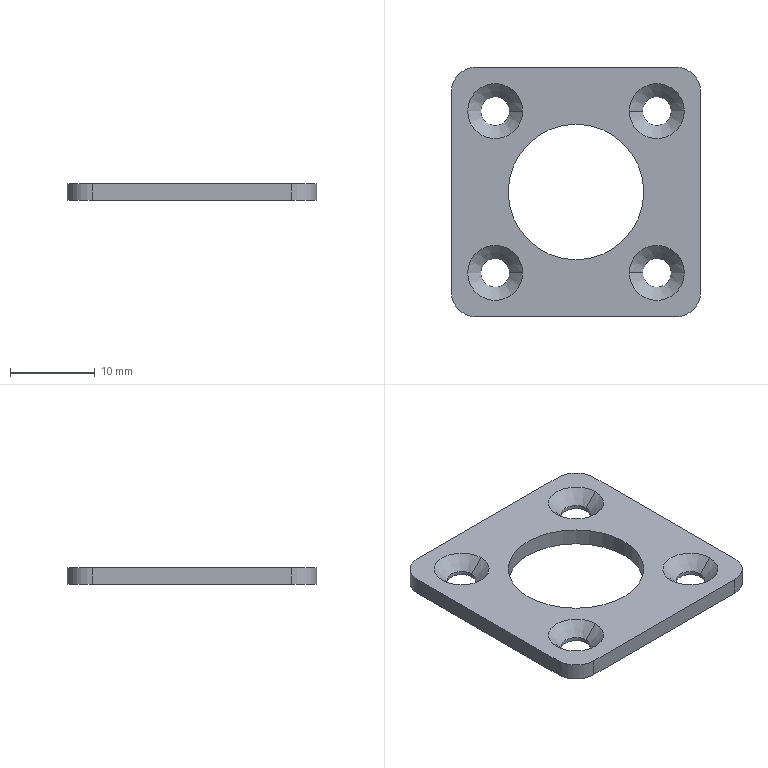Part | NX | features BREP 1 | 1 solid | 28 faces | box 29.5 x 29.5 x 2 mm | volume 1183 mm3 | cylinder 14 | cone 8 | plane 6 | commonest cylinder face diameters 3.4 x8 6 x4 16 x2
STEP:
#1=CARTESIAN_POINT('',(6.296,9.546,2.));
#2=VERTEX_POINT('',#1);
#3=CARTESIAN_POINT('',(7.846,9.546,0.45));
#4=VERTEX_POINT('',#3);
#5=CARTESIAN_POINT('',(6.296,9.546,2.));
#6=DIRECTION('',(-0.7071,0.,0.7071));
#7=VECTOR('',#6,1000.);
#8=LINE('',#5,#7);
#9=EDGE_CURVE('',#2,#4,#8,.F.);
#10=ORIENTED_EDGE('',*,*,#9,.T.);
#11=CARTESIAN_POINT('',(11.246,9.546,0.45));
#12=VERTEX_POINT('',#11);
#13=CARTESIAN_POINT('',(9.546,9.546,0.45));
#14=DIRECTION('',(0.,0.,1.));
#15=DIRECTION('',(1.,0.,0.));
#16=AXIS2_PLACEMENT_3D('',#13,#14,#15);
#17=CIRCLE('',#16,1.7);
#18=EDGE_CURVE('',#12,#4,#17,.T.);
#19=ORIENTED_EDGE('',*,*,#18,.F.);
#20=CARTESIAN_POINT('',(12.796,9.546,2.));
#21=VERTEX_POINT('',#20);
#22=CARTESIAN_POINT('',(12.796,9.546,2.));
#23=DIRECTION('',(0.7071,0.,0.7071));
#24=VECTOR('',#23,1000.);
#25=LINE('',#22,#24);
#26=EDGE_CURVE('',#21,#12,#25,.F.);
#27=ORIENTED_EDGE('',*,*,#26,.F.);
#28=CARTESIAN_POINT('',(9.546,9.546,2.));
#29=DIRECTION('',(0.,0.,1.));
#30=DIRECTION('',(1.,0.,0.));
#31=AXIS2_PLACEMENT_3D('',#28,#29,#30);
#32=CIRCLE('',#31,3.25);
#33=EDGE_CURVE('',#21,#2,#32,.T.);
#34=ORIENTED_EDGE('',*,*,#33,.T.);
#35=EDGE_LOOP('',(#10,#19,#27,#34));
#36=FACE_BOUND('',#35,.T.);
#37=CARTESIAN_POINT('',(9.546,9.546,2.));
#38=DIRECTION('',(0.,0.,1.));
#39=DIRECTION('',(1.,0.,0.));
#40=AXIS2_PLACEMENT_3D('',#37,#38,#39);
#41=CONICAL_SURFACE('',#40,3.25,0.7854);
#42=ADVANCED_FACE('',(#36),#41,.F.);
#43=CARTESIAN_POINT('',(7.846,9.546,0.));
#44=VERTEX_POINT('',#43);
#45=CARTESIAN_POINT('',(7.846,9.546,2.));
#46=DIRECTION('',(0.,0.,1.));
#47=VECTOR('',#46,1000.);
#48=LINE('',#45,#47);
#49=EDGE_CURVE('',#4,#44,#48,.F.);
#50=ORIENTED_EDGE('',*,*,#49,.T.);
#51=CARTESIAN_POINT('',(11.246,9.546,0.));
#52=VERTEX_POINT('',#51);
#53=CARTESIAN_POINT('',(9.546,9.546,0.));
#54=DIRECTION('',(0.,0.,-1.));
#55=DIRECTION('',(-1.,0.,0.));
#56=AXIS2_PLACEMENT_3D('',#53,#54,#55);
#57=CIRCLE('',#56,1.7);
#58=EDGE_CURVE('',#44,#52,#57,.T.);
#59=ORIENTED_EDGE('',*,*,#58,.T.);
#60=CARTESIAN_POINT('',(11.246,9.546,2.));
#61=DIRECTION('',(0.,0.,1.));
#62=VECTOR('',#61,1000.);
#63=LINE('',#60,#62);
#64=EDGE_CURVE('',#12,#52,#63,.F.);
#65=ORIENTED_EDGE('',*,*,#64,.F.);
#66=ORIENTED_EDGE('',*,*,#18,.T.);
#67=EDGE_LOOP('',(#50,#59,#65,#66));
#68=FACE_BOUND('',#67,.T.);
#69=CARTESIAN_POINT('',(9.546,9.546,2.));
#70=DIRECTION('',(0.,0.,1.));
#71=DIRECTION('',(1.,0.,0.));
#72=AXIS2_PLACEMENT_3D('',#69,#70,#71);
#73=CYLINDRICAL_SURFACE('',#72,1.7);
#74=ADVANCED_FACE('',(#68),#73,.F.);
#75=CARTESIAN_POINT('',(6.296,-9.546,2.));
#76=VERTEX_POINT('',#75);
#77=CARTESIAN_POINT('',(7.846,-9.546,0.45));
#78=VERTEX_POINT('',#77);
#79=CARTESIAN_POINT('',(6.296,-9.546,2.));
#80=DIRECTION('',(-0.7071,0.,0.7071));
#81=VECTOR('',#80,1000.);
#82=LINE('',#79,#81);
#83=EDGE_CURVE('',#76,#78,#82,.F.);
#84=ORIENTED_EDGE('',*,*,#83,.T.);
#85=CARTESIAN_POINT('',(11.246,-9.546,0.45));
#86=VERTEX_POINT('',#85);
#87=CARTESIAN_POINT('',(9.546,-9.546,0.45));
#88=DIRECTION('',(0.,0.,1.));
#89=DIRECTION('',(1.,0.,0.));
#90=AXIS2_PLACEMENT_3D('',#87,#88,#89);
#91=CIRCLE('',#90,1.7);
#92=EDGE_CURVE('',#86,#78,#91,.T.);
#93=ORIENTED_EDGE('',*,*,#92,.F.);
#94=CARTESIAN_POINT('',(12.796,-9.546,2.));
#95=VERTEX_POINT('',#94);
#96=CARTESIAN_POINT('',(12.796,-9.546,2.));
#97=DIRECTION('',(0.7071,0.,0.7071));
#98=VECTOR('',#97,1000.);
#99=LINE('',#96,#98);
#100=EDGE_CURVE('',#95,#86,#99,.F.);
#101=ORIENTED_EDGE('',*,*,#100,.F.);
#102=CARTESIAN_POINT('',(9.546,-9.546,2.));
#103=DIRECTION('',(0.,0.,1.));
#104=DIRECTION('',(1.,0.,0.));
#105=AXIS2_PLACEMENT_3D('',#102,#103,#104);
#106=CIRCLE('',#105,3.25);
#107=EDGE_CURVE('',#95,#76,#106,.T.);
#108=ORIENTED_EDGE('',*,*,#107,.T.);
#109=EDGE_LOOP('',(#84,#93,#101,#108));
#110=FACE_BOUND('',#109,.T.);
#111=CARTESIAN_POINT('',(9.546,-9.546,2.));
#112=DIRECTION('',(0.,0.,1.));
#113=DIRECTION('',(1.,0.,0.));
#114=AXIS2_PLACEMENT_3D('',#111,#112,#113);
#115=CONICAL_SURFACE('',#114,3.25,0.7854);
#116=ADVANCED_FACE('',(#110),#115,.F.);
#117=CARTESIAN_POINT('',(7.846,-9.546,0.));
#118=VERTEX_POINT('',#117);
#119=CARTESIAN_POINT('',(7.846,-9.546,2.));
#120=DIRECTION('',(0.,0.,1.));
#121=VECTOR('',#120,1000.);
#122=LINE('',#119,#121);
#123=EDGE_CURVE('',#78,#118,#122,.F.);
#124=ORIENTED_EDGE('',*,*,#123,.T.);
#125=CARTESIAN_POINT('',(11.246,-9.546,0.));
#126=VERTEX_POINT('',#125);
#127=CARTESIAN_POINT('',(9.546,-9.546,0.));
#128=DIRECTION('',(0.,0.,-1.));
#129=DIRECTION('',(-1.,0.,0.));
#130=AXIS2_PLACEMENT_3D('',#127,#128,#129);
#131=CIRCLE('',#130,1.7);
#132=EDGE_CURVE('',#118,#126,#131,.T.);
#133=ORIENTED_EDGE('',*,*,#132,.T.);
#134=CARTESIAN_POINT('',(11.246,-9.546,2.));
#135=DIRECTION('',(0.,0.,1.));
#136=VECTOR('',#135,1000.);
#137=LINE('',#134,#136);
#138=EDGE_CURVE('',#86,#126,#137,.F.);
#139=ORIENTED_EDGE('',*,*,#138,.F.);
#140=ORIENTED_EDGE('',*,*,#92,.T.);
#141=EDGE_LOOP('',(#124,#133,#139,#140));
#142=FACE_BOUND('',#141,.T.);
#143=CARTESIAN_POINT('',(9.546,-9.546,2.));
#144=DIRECTION('',(0.,0.,1.));
#145=DIRECTION('',(1.,0.,0.));
#146=AXIS2_PLACEMENT_3D('',#143,#144,#145);
#147=CYLINDRICAL_SURFACE('',#146,1.7);
#148=ADVANCED_FACE('',(#142),#147,.F.);
#149=CARTESIAN_POINT('',(-12.796,-9.546,2.));
#150=VERTEX_POINT('',#149);
#151=CARTESIAN_POINT('',(-11.246,-9.546,0.45));
#152=VERTEX_POINT('',#151);
#153=CARTESIAN_POINT('',(-12.796,-9.546,2.));
#154=DIRECTION('',(-0.7071,0.,0.7071));
#155=VECTOR('',#154,1000.);
#156=LINE('',#153,#155);
#157=EDGE_CURVE('',#150,#152,#156,.F.);
#158=ORIENTED_EDGE('',*,*,#157,.T.);
#159=CARTESIAN_POINT('',(-7.846,-9.546,0.45));
#160=VERTEX_POINT('',#159);
#161=CARTESIAN_POINT('',(-9.546,-9.546,0.45));
#162=DIRECTION('',(0.,0.,1.));
#163=DIRECTION('',(1.,0.,0.));
#164=AXIS2_PLACEMENT_3D('',#161,#162,#163);
#165=CIRCLE('',#164,1.7);
#166=EDGE_CURVE('',#160,#152,#165,.T.);
#167=ORIENTED_EDGE('',*,*,#166,.F.);
#168=CARTESIAN_POINT('',(-6.296,-9.546,2.));
#169=VERTEX_POINT('',#168);
#170=CARTESIAN_POINT('',(-6.296,-9.546,2.));
#171=DIRECTION('',(0.7071,0.,0.7071));
#172=VECTOR('',#171,1000.);
#173=LINE('',#170,#172);
#174=EDGE_CURVE('',#169,#160,#173,.F.);
#175=ORIENTED_EDGE('',*,*,#174,.F.);
#176=CARTESIAN_POINT('',(-9.546,-9.546,2.));
#177=DIRECTION('',(0.,0.,1.));
#178=DIRECTION('',(1.,0.,0.));
#179=AXIS2_PLACEMENT_3D('',#176,#177,#178);
#180=CIRCLE('',#179,3.25);
#181=EDGE_CURVE('',#169,#150,#180,.T.);
#182=ORIENTED_EDGE('',*,*,#181,.T.);
#183=EDGE_LOOP('',(#158,#167,#175,#182));
#184=FACE_BOUND('',#183,.T.);
#185=CARTESIAN_POINT('',(-9.546,-9.546,2.));
#186=DIRECTION('',(0.,0.,1.));
#187=DIRECTION('',(1.,0.,0.));
#188=AXIS2_PLACEMENT_3D('',#185,#186,#187);
#189=CONICAL_SURFACE('',#188,3.25,0.7854);
#190=ADVANCED_FACE('',(#184),#189,.F.);
#191=CARTESIAN_POINT('',(-11.246,-9.546,0.));
#192=VERTEX_POINT('',#191);
#193=CARTESIAN_POINT('',(-11.246,-9.546,2.));
#194=DIRECTION('',(0.,0.,1.));
#195=VECTOR('',#194,1000.);
#196=LINE('',#193,#195);
#197=EDGE_CURVE('',#152,#192,#196,.F.);
#198=ORIENTED_EDGE('',*,*,#197,.T.);
#199=CARTESIAN_POINT('',(-7.846,-9.546,0.));
#200=VERTEX_POINT('',#199);
#201=CARTESIAN_POINT('',(-9.546,-9.546,0.));
#202=DIRECTION('',(0.,0.,-1.));
#203=DIRECTION('',(-1.,0.,0.));
#204=AXIS2_PLACEMENT_3D('',#201,#202,#203);
#205=CIRCLE('',#204,1.7);
#206=EDGE_CURVE('',#192,#200,#205,.T.);
#207=ORIENTED_EDGE('',*,*,#206,.T.);
#208=CARTESIAN_POINT('',(-7.846,-9.546,2.));
#209=DIRECTION('',(0.,0.,1.));
#210=VECTOR('',#209,1000.);
#211=LINE('',#208,#210);
#212=EDGE_CURVE('',#160,#200,#211,.F.);
#213=ORIENTED_EDGE('',*,*,#212,.F.);
#214=ORIENTED_EDGE('',*,*,#166,.T.);
#215=EDGE_LOOP('',(#198,#207,#213,#214));
#216=FACE_BOUND('',#215,.T.);
#217=CARTESIAN_POINT('',(-9.546,-9.546,2.));
#218=DIRECTION('',(0.,0.,1.));
#219=DIRECTION('',(1.,0.,0.));
#220=AXIS2_PLACEMENT_3D('',#217,#218,#219);
#221=CYLINDRICAL_SURFACE('',#220,1.7);
#222=ADVANCED_FACE('',(#216),#221,.F.);
#223=CARTESIAN_POINT('',(-12.796,9.546,2.));
#224=VERTEX_POINT('',#223);
#225=CARTESIAN_POINT('',(-11.246,9.546,0.45));
#226=VERTEX_POINT('',#225);
#227=CARTESIAN_POINT('',(-12.796,9.546,2.));
#228=DIRECTION('',(-0.7071,0.,0.7071));
#229=VECTOR('',#228,1000.);
#230=LINE('',#227,#229);
#231=EDGE_CURVE('',#224,#226,#230,.F.);
#232=ORIENTED_EDGE('',*,*,#231,.T.);
#233=CARTESIAN_POINT('',(-7.846,9.546,0.45));
#234=VERTEX_POINT('',#233);
#235=CARTESIAN_POINT('',(-9.546,9.546,0.45));
#236=DIRECTION('',(0.,0.,1.));
#237=DIRECTION('',(1.,0.,0.));
#238=AXIS2_PLACEMENT_3D('',#235,#236,#237);
#239=CIRCLE('',#238,1.7);
#240=EDGE_CURVE('',#234,#226,#239,.T.);
#241=ORIENTED_EDGE('',*,*,#240,.F.);
#242=CARTESIAN_POINT('',(-6.296,9.546,2.));
#243=VERTEX_POINT('',#242);
#244=CARTESIAN_POINT('',(-6.296,9.546,2.));
#245=DIRECTION('',(0.7071,0.,0.7071));
#246=VECTOR('',#245,1000.);
#247=LINE('',#244,#246);
#248=EDGE_CURVE('',#243,#234,#247,.F.);
#249=ORIENTED_EDGE('',*,*,#248,.F.);
#250=CARTESIAN_POINT('',(-9.546,9.546,2.));
#251=DIRECTION('',(0.,0.,1.));
#252=DIRECTION('',(1.,0.,0.));
#253=AXIS2_PLACEMENT_3D('',#250,#251,#252);
#254=CIRCLE('',#253,3.25);
#255=EDGE_CURVE('',#243,#224,#254,.T.);
#256=ORIENTED_EDGE('',*,*,#255,.T.);
#257=EDGE_LOOP('',(#232,#241,#249,#256));
#258=FACE_BOUND('',#257,.T.);
#259=CARTESIAN_POINT('',(-9.546,9.546,2.));
#260=DIRECTION('',(0.,0.,1.));
#261=DIRECTION('',(1.,0.,0.));
#262=AXIS2_PLACEMENT_3D('',#259,#260,#261);
#263=CONICAL_SURFACE('',#262,3.25,0.7854);
#264=ADVANCED_FACE('',(#258),#263,.F.);
#265=CARTESIAN_POINT('',(-11.246,9.546,0.));
#266=VERTEX_POINT('',#265);
#267=CARTESIAN_POINT('',(-11.246,9.546,2.));
#268=DIRECTION('',(0.,0.,1.));
#269=VECTOR('',#268,1000.);
#270=LINE('',#267,#269);
#271=EDGE_CURVE('',#226,#266,#270,.F.);
#272=ORIENTED_EDGE('',*,*,#271,.T.);
#273=CARTESIAN_POINT('',(-7.846,9.546,0.));
#274=VERTEX_POINT('',#273);
#275=CARTESIAN_POINT('',(-9.546,9.546,0.));
#276=DIRECTION('',(0.,0.,-1.));
#277=DIRECTION('',(-1.,0.,0.));
#278=AXIS2_PLACEMENT_3D('',#275,#276,#277);
#279=CIRCLE('',#278,1.7);
#280=EDGE_CURVE('',#266,#274,#279,.T.);
#281=ORIENTED_EDGE('',*,*,#280,.T.);
#282=CARTESIAN_POINT('',(-7.846,9.546,2.));
#283=DIRECTION('',(0.,0.,1.));
#284=VECTOR('',#283,1000.);
#285=LINE('',#282,#284);
#286=EDGE_CURVE('',#234,#274,#285,.F.);
#287=ORIENTED_EDGE('',*,*,#286,.F.);
#288=ORIENTED_EDGE('',*,*,#240,.T.);
#289=EDGE_LOOP('',(#272,#281,#287,#288));
#290=FACE_BOUND('',#289,.T.);
#291=CARTESIAN_POINT('',(-9.546,9.546,2.));
#292=DIRECTION('',(0.,0.,1.));
#293=DIRECTION('',(1.,0.,0.));
#294=AXIS2_PLACEMENT_3D('',#291,#292,#293);
#295=CYLINDRICAL_SURFACE('',#294,1.7);
#296=ADVANCED_FACE('',(#290),#295,.F.);
#297=CARTESIAN_POINT('',(14.75,11.75,2.));
#298=VERTEX_POINT('',#297);
#299=CARTESIAN_POINT('',(11.75,14.75,2.));
#300=VERTEX_POINT('',#299);
#301=CARTESIAN_POINT('',(11.75,11.75,2.));
#302=DIRECTION('',(0.,0.,1.));
#303=DIRECTION('',(-1.,0.,0.));
#304=AXIS2_PLACEMENT_3D('',#301,#302,#303);
#305=CIRCLE('',#304,3.);
#306=EDGE_CURVE('',#298,#300,#305,.T.);
#307=ORIENTED_EDGE('',*,*,#306,.F.);
#308=CARTESIAN_POINT('',(14.75,11.75,0.));
#309=VERTEX_POINT('',#308);
#310=CARTESIAN_POINT('',(14.75,11.75,2.));
#311=DIRECTION('',(0.,0.,1.));
#312=VECTOR('',#311,1000.);
#313=LINE('',#310,#312);
#314=EDGE_CURVE('',#309,#298,#313,.T.);
#315=ORIENTED_EDGE('',*,*,#314,.F.);
#316=CARTESIAN_POINT('',(11.75,14.75,0.));
#317=VERTEX_POINT('',#316);
#318=CARTESIAN_POINT('',(11.75,11.75,0.));
#319=DIRECTION('',(0.,0.,-1.));
#320=DIRECTION('',(-1.,0.,0.));
#321=AXIS2_PLACEMENT_3D('',#318,#319,#320);
#322=CIRCLE('',#321,3.);
#323=EDGE_CURVE('',#317,#309,#322,.T.);
#324=ORIENTED_EDGE('',*,*,#323,.F.);
#325=CARTESIAN_POINT('',(11.75,14.75,2.));
#326=DIRECTION('',(0.,0.,-1.));
#327=VECTOR('',#326,1000.);
#328=LINE('',#325,#327);
#329=EDGE_CURVE('',#300,#317,#328,.T.);
#330=ORIENTED_EDGE('',*,*,#329,.F.);
#331=EDGE_LOOP('',(#307,#315,#324,#330));
#332=FACE_BOUND('',#331,.T.);
#333=CARTESIAN_POINT('',(11.75,11.75,2.));
#334=DIRECTION('',(0.,0.,-1.));
#335=DIRECTION('',(-1.,0.,0.));
#336=AXIS2_PLACEMENT_3D('',#333,#334,#335);
#337=CYLINDRICAL_SURFACE('',#336,3.);
#338=ADVANCED_FACE('',(#332),#337,.T.);
#339=CARTESIAN_POINT('',(-11.75,14.75,2.));
#340=VERTEX_POINT('',#339);
#341=CARTESIAN_POINT('',(-14.75,11.75,2.));
#342=VERTEX_POINT('',#341);
#343=CARTESIAN_POINT('',(-11.75,11.75,2.));
#344=DIRECTION('',(0.,0.,1.));
#345=DIRECTION('',(-1.,0.,0.));
#346=AXIS2_PLACEMENT_3D('',#343,#344,#345);
#347=CIRCLE('',#346,3.);
#348=EDGE_CURVE('',#340,#342,#347,.T.);
#349=ORIENTED_EDGE('',*,*,#348,.F.);
#350=CARTESIAN_POINT('',(-11.75,14.75,0.));
#351=VERTEX_POINT('',#350);
#352=CARTESIAN_POINT('',(-11.75,14.75,2.));
#353=DIRECTION('',(0.,0.,1.));
#354=VECTOR('',#353,1000.);
#355=LINE('',#352,#354);
#356=EDGE_CURVE('',#351,#340,#355,.T.);
#357=ORIENTED_EDGE('',*,*,#356,.F.);
#358=CARTESIAN_POINT('',(-14.75,11.75,0.));
#359=VERTEX_POINT('',#358);
#360=CARTESIAN_POINT('',(-11.75,11.75,0.));
#361=DIRECTION('',(0.,0.,-1.));
#362=DIRECTION('',(-1.,0.,0.));
#363=AXIS2_PLACEMENT_3D('',#360,#361,#362);
#364=CIRCLE('',#363,3.);
#365=EDGE_CURVE('',#359,#351,#364,.T.);
#366=ORIENTED_EDGE('',*,*,#365,.F.);
#367=CARTESIAN_POINT('',(-14.75,11.75,2.));
#368=DIRECTION('',(0.,0.,-1.));
#369=VECTOR('',#368,1000.);
#370=LINE('',#367,#369);
#371=EDGE_CURVE('',#342,#359,#370,.T.);
#372=ORIENTED_EDGE('',*,*,#371,.F.);
#373=EDGE_LOOP('',(#349,#357,#366,#372));
#374=FACE_BOUND('',#373,.T.);
#375=CARTESIAN_POINT('',(-11.75,11.75,2.));
#376=DIRECTION('',(0.,0.,-1.));
#377=DIRECTION('',(-1.,0.,0.));
#378=AXIS2_PLACEMENT_3D('',#375,#376,#377);
#379=CYLINDRICAL_SURFACE('',#378,3.);
#380=ADVANCED_FACE('',(#374),#379,.T.);
#381=CARTESIAN_POINT('',(11.75,-14.75,2.));
#382=VERTEX_POINT('',#381);
#383=CARTESIAN_POINT('',(14.75,-11.75,2.));
#384=VERTEX_POINT('',#383);
#385=CARTESIAN_POINT('',(11.75,-11.75,2.));
#386=DIRECTION('',(0.,0.,1.));
#387=DIRECTION('',(-1.,0.,0.));
#388=AXIS2_PLACEMENT_3D('',#385,#386,#387);
#389=CIRCLE('',#388,3.);
#390=EDGE_CURVE('',#382,#384,#389,.T.);
#391=ORIENTED_EDGE('',*,*,#390,.F.);
#392=CARTESIAN_POINT('',(11.75,-14.75,0.));
#393=VERTEX_POINT('',#392);
#394=CARTESIAN_POINT('',(11.75,-14.75,2.));
#395=DIRECTION('',(0.,0.,1.));
#396=VECTOR('',#395,1000.);
#397=LINE('',#394,#396);
#398=EDGE_CURVE('',#393,#382,#397,.T.);
#399=ORIENTED_EDGE('',*,*,#398,.F.);
#400=CARTESIAN_POINT('',(14.75,-11.75,0.));
#401=VERTEX_POINT('',#400);
#402=CARTESIAN_POINT('',(11.75,-11.75,0.));
#403=DIRECTION('',(0.,0.,-1.));
#404=DIRECTION('',(-1.,0.,0.));
#405=AXIS2_PLACEMENT_3D('',#402,#403,#404);
#406=CIRCLE('',#405,3.);
#407=EDGE_CURVE('',#401,#393,#406,.T.);
#408=ORIENTED_EDGE('',*,*,#407,.F.);
#409=CARTESIAN_POINT('',(14.75,-11.75,2.));
#410=DIRECTION('',(0.,0.,-1.));
#411=VECTOR('',#410,1000.);
#412=LINE('',#409,#411);
#413=EDGE_CURVE('',#384,#401,#412,.T.);
#414=ORIENTED_EDGE('',*,*,#413,.F.);
#415=EDGE_LOOP('',(#391,#399,#408,#414));
#416=FACE_BOUND('',#415,.T.);
#417=CARTESIAN_POINT('',(11.75,-11.75,2.));
#418=DIRECTION('',(0.,0.,-1.));
#419=DIRECTION('',(-1.,0.,0.));
#420=AXIS2_PLACEMENT_3D('',#417,#418,#419);
#421=CYLINDRICAL_SURFACE('',#420,3.);
#422=ADVANCED_FACE('',(#416),#421,.T.);
#423=CARTESIAN_POINT('',(-14.75,-11.75,2.));
#424=VERTEX_POINT('',#423);
#425=CARTESIAN_POINT('',(-11.75,-14.75,2.));
#426=VERTEX_POINT('',#425);
#427=CARTESIAN_POINT('',(-11.75,-11.75,2.));
#428=DIRECTION('',(0.,0.,1.));
#429=DIRECTION('',(-1.,0.,0.));
#430=AXIS2_PLACEMENT_3D('',#427,#428,#429);
#431=CIRCLE('',#430,3.);
#432=EDGE_CURVE('',#424,#426,#431,.T.);
#433=ORIENTED_EDGE('',*,*,#432,.F.);
#434=CARTESIAN_POINT('',(-14.75,-11.75,0.));
#435=VERTEX_POINT('',#434);
#436=CARTESIAN_POINT('',(-14.75,-11.75,2.));
#437=DIRECTION('',(0.,0.,1.));
#438=VECTOR('',#437,1000.);
#439=LINE('',#436,#438);
#440=EDGE_CURVE('',#435,#424,#439,.T.);
#441=ORIENTED_EDGE('',*,*,#440,.F.);
#442=CARTESIAN_POINT('',(-11.75,-14.75,0.));
#443=VERTEX_POINT('',#442);
#444=CARTESIAN_POINT('',(-11.75,-11.75,0.));
#445=DIRECTION('',(0.,0.,-1.));
#446=DIRECTION('',(-1.,0.,0.));
#447=AXIS2_PLACEMENT_3D('',#444,#445,#446);
#448=CIRCLE('',#447,3.);
#449=EDGE_CURVE('',#443,#435,#448,.T.);
#450=ORIENTED_EDGE('',*,*,#449,.F.);
#451=CARTESIAN_POINT('',(-11.75,-14.75,2.));
#452=DIRECTION('',(0.,0.,-1.));
#453=VECTOR('',#452,1000.);
#454=LINE('',#451,#453);
#455=EDGE_CURVE('',#426,#443,#454,.T.);
#456=ORIENTED_EDGE('',*,*,#455,.F.);
#457=EDGE_LOOP('',(#433,#441,#450,#456));
#458=FACE_BOUND('',#457,.T.);
#459=CARTESIAN_POINT('',(-11.75,-11.75,2.));
#460=DIRECTION('',(0.,0.,-1.));
#461=DIRECTION('',(-1.,0.,0.));
#462=AXIS2_PLACEMENT_3D('',#459,#460,#461);
#463=CYLINDRICAL_SURFACE('',#462,3.);
#464=ADVANCED_FACE('',(#458),#463,.T.);
#465=CARTESIAN_POINT('',(8.,0.,2.));
#466=VERTEX_POINT('',#465);
#467=CARTESIAN_POINT('',(8.,0.,0.));
#468=VERTEX_POINT('',#467);
#469=CARTESIAN_POINT('',(8.,0.,2.));
#470=DIRECTION('',(0.,0.,-1.));
#471=VECTOR('',#470,1000.);
#472=LINE('',#469,#471);
#473=EDGE_CURVE('',#466,#468,#472,.T.);
#474=ORIENTED_EDGE('',*,*,#473,.F.);
#475=CARTESIAN_POINT('',(-8.,0.,2.));
#476=VERTEX_POINT('',#475);
#477=CARTESIAN_POINT('',(0.,0.,2.));
#478=DIRECTION('',(0.,0.,1.));
#479=DIRECTION('',(1.,0.,0.));
#480=AXIS2_PLACEMENT_3D('',#477,#478,#479);
#481=CIRCLE('',#480,8.);
#482=EDGE_CURVE('',#466,#476,#481,.T.);
#483=ORIENTED_EDGE('',*,*,#482,.T.);
#484=CARTESIAN_POINT('',(-8.,0.,0.));
#485=VERTEX_POINT('',#484);
#486=CARTESIAN_POINT('',(-8.,0.,2.));
#487=DIRECTION('',(0.,0.,-1.));
#488=VECTOR('',#487,1000.);
#489=LINE('',#486,#488);
#490=EDGE_CURVE('',#476,#485,#489,.T.);
#491=ORIENTED_EDGE('',*,*,#490,.T.);
#492=CARTESIAN_POINT('',(0.,0.,0.));
#493=DIRECTION('',(0.,0.,1.));
#494=DIRECTION('',(1.,0.,0.));
#495=AXIS2_PLACEMENT_3D('',#492,#493,#494);
#496=CIRCLE('',#495,8.);
#497=EDGE_CURVE('',#468,#485,#496,.T.);
#498=ORIENTED_EDGE('',*,*,#497,.F.);
#499=EDGE_LOOP('',(#474,#483,#491,#498));
#500=FACE_BOUND('',#499,.T.);
#501=CARTESIAN_POINT('',(0.,0.,2.));
#502=DIRECTION('',(0.,0.,-1.));
#503=DIRECTION('',(-1.,0.,0.));
#504=AXIS2_PLACEMENT_3D('',#501,#502,#503);
#505=CYLINDRICAL_SURFACE('',#504,8.);
#506=ADVANCED_FACE('',(#500),#505,.F.);
#507=CARTESIAN_POINT('',(14.75,14.75,0.));
#508=DIRECTION('',(-1.,0.,0.));
#509=VECTOR('',#508,1000.);
#510=LINE('',#507,#509);
#511=EDGE_CURVE('',#317,#351,#510,.T.);
#512=ORIENTED_EDGE('',*,*,#511,.T.);
#513=ORIENTED_EDGE('',*,*,#356,.T.);
#514=CARTESIAN_POINT('',(14.75,14.75,2.));
#515=DIRECTION('',(-1.,0.,0.));
#516=VECTOR('',#515,1000.);
#517=LINE('',#514,#516);
#518=EDGE_CURVE('',#300,#340,#517,.T.);
#519=ORIENTED_EDGE('',*,*,#518,.F.);
#520=ORIENTED_EDGE('',*,*,#329,.T.);
#521=EDGE_LOOP('',(#512,#513,#519,#520));
#522=FACE_BOUND('',#521,.T.);
#523=CARTESIAN_POINT('',(14.75,14.75,2.));
#524=DIRECTION('',(0.,-1.,0.));
#525=DIRECTION('',(1.,0.,0.));
#526=AXIS2_PLACEMENT_3D('',#523,#524,#525);
#527=PLANE('',#526);
#528=ADVANCED_FACE('',(#522),#527,.F.);
#529=CARTESIAN_POINT('',(14.75,14.75,2.));
#530=DIRECTION('',(0.,1.,0.));
#531=VECTOR('',#530,1000.);
#532=LINE('',#529,#531);
#533=EDGE_CURVE('',#384,#298,#532,.T.);
#534=ORIENTED_EDGE('',*,*,#533,.F.);
#535=ORIENTED_EDGE('',*,*,#413,.T.);
#536=CARTESIAN_POINT('',(14.75,14.75,0.));
#537=DIRECTION('',(0.,1.,0.));
#538=VECTOR('',#537,1000.);
#539=LINE('',#536,#538);
#540=EDGE_CURVE('',#401,#309,#539,.T.);
#541=ORIENTED_EDGE('',*,*,#540,.T.);
#542=ORIENTED_EDGE('',*,*,#314,.T.);
#543=EDGE_LOOP('',(#534,#535,#541,#542));
#544=FACE_BOUND('',#543,.T.);
#545=CARTESIAN_POINT('',(14.75,14.75,2.));
#546=DIRECTION('',(-1.,0.,0.));
#547=DIRECTION('',(0.,-1.,0.));
#548=AXIS2_PLACEMENT_3D('',#545,#546,#547);
#549=PLANE('',#548);
#550=ADVANCED_FACE('',(#544),#549,.F.);
#551=CARTESIAN_POINT('',(14.75,-14.75,2.));
#552=DIRECTION('',(1.,0.,0.));
#553=VECTOR('',#552,1000.);
#554=LINE('',#551,#553);
#555=EDGE_CURVE('',#426,#382,#554,.T.);
#556=ORIENTED_EDGE('',*,*,#555,.F.);
#557=ORIENTED_EDGE('',*,*,#455,.T.);
#558=CARTESIAN_POINT('',(14.75,-14.75,0.));
#559=DIRECTION('',(1.,0.,0.));
#560=VECTOR('',#559,1000.);
#561=LINE('',#558,#560);
#562=EDGE_CURVE('',#443,#393,#561,.T.);
#563=ORIENTED_EDGE('',*,*,#562,.T.);
#564=ORIENTED_EDGE('',*,*,#398,.T.);
#565=EDGE_LOOP('',(#556,#557,#563,#564));
#566=FACE_BOUND('',#565,.T.);
#567=CARTESIAN_POINT('',(14.75,-14.75,2.));
#568=DIRECTION('',(0.,1.,0.));
#569=DIRECTION('',(-1.,0.,0.));
#570=AXIS2_PLACEMENT_3D('',#567,#568,#569);
#571=PLANE('',#570);
#572=ADVANCED_FACE('',(#566),#571,.F.);
#573=CARTESIAN_POINT('',(-14.75,14.75,0.));
#574=DIRECTION('',(0.,-1.,0.));
#575=VECTOR('',#574,1000.);
#576=LINE('',#573,#575);
#577=EDGE_CURVE('',#359,#435,#576,.T.);
#578=ORIENTED_EDGE('',*,*,#577,.T.);
#579=ORIENTED_EDGE('',*,*,#440,.T.);
#580=CARTESIAN_POINT('',(-14.75,14.75,2.));
#581=DIRECTION('',(0.,-1.,0.));
#582=VECTOR('',#581,1000.);
#583=LINE('',#580,#582);
#584=EDGE_CURVE('',#342,#424,#583,.T.);
#585=ORIENTED_EDGE('',*,*,#584,.F.);
#586=ORIENTED_EDGE('',*,*,#371,.T.);
#587=EDGE_LOOP('',(#578,#579,#585,#586));
#588=FACE_BOUND('',#587,.T.);
#589=CARTESIAN_POINT('',(-14.75,14.75,2.));
#590=DIRECTION('',(1.,0.,0.));
#591=DIRECTION('',(0.,1.,0.));
#592=AXIS2_PLACEMENT_3D('',#589,#590,#591);
#593=PLANE('',#592);
#594=ADVANCED_FACE('',(#588),#593,.F.);
#595=CARTESIAN_POINT('',(0.,0.,0.));
#596=DIRECTION('',(0.,0.,1.));
#597=DIRECTION('',(1.,0.,0.));
#598=AXIS2_PLACEMENT_3D('',#595,#596,#597);
#599=CIRCLE('',#598,8.);
#600=EDGE_CURVE('',#485,#468,#599,.T.);
#601=ORIENTED_EDGE('',*,*,#600,.T.);
#602=ORIENTED_EDGE('',*,*,#497,.T.);
#603=EDGE_LOOP('',(#601,#602));
#604=FACE_BOUND('',#603,.T.);
#605=ORIENTED_EDGE('',*,*,#562,.F.);
#606=ORIENTED_EDGE('',*,*,#449,.T.);
#607=ORIENTED_EDGE('',*,*,#577,.F.);
#608=ORIENTED_EDGE('',*,*,#365,.T.);
#609=ORIENTED_EDGE('',*,*,#511,.F.);
#610=ORIENTED_EDGE('',*,*,#323,.T.);
#611=ORIENTED_EDGE('',*,*,#540,.F.);
#612=ORIENTED_EDGE('',*,*,#407,.T.);
#613=EDGE_LOOP('',(#605,#606,#607,#608,#609,#610,#611,#612));
#614=FACE_BOUND('',#613,.T.);
#615=CARTESIAN_POINT('',(-9.546,9.546,0.));
#616=DIRECTION('',(0.,0.,-1.));
#617=DIRECTION('',(-1.,0.,0.));
#618=AXIS2_PLACEMENT_3D('',#615,#616,#617);
#619=CIRCLE('',#618,1.7);
#620=EDGE_CURVE('',#274,#266,#619,.T.);
#621=ORIENTED_EDGE('',*,*,#620,.F.);
#622=ORIENTED_EDGE('',*,*,#280,.F.);
#623=EDGE_LOOP('',(#621,#622));
#624=FACE_BOUND('',#623,.T.);
#625=CARTESIAN_POINT('',(-9.546,-9.546,0.));
#626=DIRECTION('',(0.,0.,-1.));
#627=DIRECTION('',(-1.,0.,0.));
#628=AXIS2_PLACEMENT_3D('',#625,#626,#627);
#629=CIRCLE('',#628,1.7);
#630=EDGE_CURVE('',#200,#192,#629,.T.);
#631=ORIENTED_EDGE('',*,*,#630,.F.);
#632=ORIENTED_EDGE('',*,*,#206,.F.);
#633=EDGE_LOOP('',(#631,#632));
#634=FACE_BOUND('',#633,.T.);
#635=CARTESIAN_POINT('',(9.546,-9.546,0.));
#636=DIRECTION('',(0.,0.,-1.));
#637=DIRECTION('',(-1.,0.,0.));
#638=AXIS2_PLACEMENT_3D('',#635,#636,#637);
#639=CIRCLE('',#638,1.7);
#640=EDGE_CURVE('',#126,#118,#639,.T.);
#641=ORIENTED_EDGE('',*,*,#640,.F.);
#642=ORIENTED_EDGE('',*,*,#132,.F.);
#643=EDGE_LOOP('',(#641,#642));
#644=FACE_BOUND('',#643,.T.);
#645=CARTESIAN_POINT('',(9.546,9.546,0.));
#646=DIRECTION('',(0.,0.,-1.));
#647=DIRECTION('',(-1.,0.,0.));
#648=AXIS2_PLACEMENT_3D('',#645,#646,#647);
#649=CIRCLE('',#648,1.7);
#650=EDGE_CURVE('',#52,#44,#649,.T.);
#651=ORIENTED_EDGE('',*,*,#650,.F.);
#652=ORIENTED_EDGE('',*,*,#58,.F.);
#653=EDGE_LOOP('',(#651,#652));
#654=FACE_BOUND('',#653,.T.);
#655=CARTESIAN_POINT('',(0.,0.,0.));
#656=DIRECTION('',(0.,0.,-1.));
#657=DIRECTION('',(-1.,0.,0.));
#658=AXIS2_PLACEMENT_3D('',#655,#656,#657);
#659=PLANE('',#658);
#660=ADVANCED_FACE('',(#604,#614,#624,#634,#644,#654),#659,.T.);
#661=ORIENTED_EDGE('',*,*,#107,.F.);
#662=CARTESIAN_POINT('',(9.546,-9.546,2.));
#663=DIRECTION('',(0.,0.,1.));
#664=DIRECTION('',(1.,0.,0.));
#665=AXIS2_PLACEMENT_3D('',#662,#663,#664);
#666=CIRCLE('',#665,3.25);
#667=EDGE_CURVE('',#76,#95,#666,.T.);
#668=ORIENTED_EDGE('',*,*,#667,.F.);
#669=EDGE_LOOP('',(#661,#668));
#670=FACE_BOUND('',#669,.T.);
#671=ORIENTED_EDGE('',*,*,#181,.F.);
#672=CARTESIAN_POINT('',(-9.546,-9.546,2.));
#673=DIRECTION('',(0.,0.,1.));
#674=DIRECTION('',(1.,0.,0.));
#675=AXIS2_PLACEMENT_3D('',#672,#673,#674);
#676=CIRCLE('',#675,3.25);
#677=EDGE_CURVE('',#150,#169,#676,.T.);
#678=ORIENTED_EDGE('',*,*,#677,.F.);
#679=EDGE_LOOP('',(#671,#678));
#680=FACE_BOUND('',#679,.T.);
#681=CARTESIAN_POINT('',(0.,0.,2.));
#682=DIRECTION('',(0.,0.,1.));
#683=DIRECTION('',(1.,0.,0.));
#684=AXIS2_PLACEMENT_3D('',#681,#682,#683);
#685=CIRCLE('',#684,8.);
#686=EDGE_CURVE('',#476,#466,#685,.T.);
#687=ORIENTED_EDGE('',*,*,#686,.F.);
#688=ORIENTED_EDGE('',*,*,#482,.F.);
#689=EDGE_LOOP('',(#687,#688));
#690=FACE_BOUND('',#689,.T.);
#691=ORIENTED_EDGE('',*,*,#584,.T.);
#692=ORIENTED_EDGE('',*,*,#432,.T.);
#693=ORIENTED_EDGE('',*,*,#555,.T.);
#694=ORIENTED_EDGE('',*,*,#390,.T.);
#695=ORIENTED_EDGE('',*,*,#533,.T.);
#696=ORIENTED_EDGE('',*,*,#306,.T.);
#697=ORIENTED_EDGE('',*,*,#518,.T.);
#698=ORIENTED_EDGE('',*,*,#348,.T.);
#699=EDGE_LOOP('',(#691,#692,#693,#694,#695,#696,#697,#698));
#700=FACE_BOUND('',#699,.T.);
#701=ORIENTED_EDGE('',*,*,#255,.F.);
#702=CARTESIAN_POINT('',(-9.546,9.546,2.));
#703=DIRECTION('',(0.,0.,1.));
#704=DIRECTION('',(1.,0.,0.));
#705=AXIS2_PLACEMENT_3D('',#702,#703,#704);
#706=CIRCLE('',#705,3.25);
#707=EDGE_CURVE('',#224,#243,#706,.T.);
#708=ORIENTED_EDGE('',*,*,#707,.F.);
#709=EDGE_LOOP('',(#701,#708));
#710=FACE_BOUND('',#709,.T.);
#711=ORIENTED_EDGE('',*,*,#33,.F.);
#712=CARTESIAN_POINT('',(9.546,9.546,2.));
#713=DIRECTION('',(0.,0.,1.));
#714=DIRECTION('',(1.,0.,0.));
#715=AXIS2_PLACEMENT_3D('',#712,#713,#714);
#716=CIRCLE('',#715,3.25);
#717=EDGE_CURVE('',#2,#21,#716,.T.);
#718=ORIENTED_EDGE('',*,*,#717,.F.);
#719=EDGE_LOOP('',(#711,#718));
#720=FACE_BOUND('',#719,.T.);
#721=CARTESIAN_POINT('',(0.,0.,2.));
#722=DIRECTION('',(0.,0.,-1.));
#723=DIRECTION('',(-1.,0.,0.));
#724=AXIS2_PLACEMENT_3D('',#721,#722,#723);
#725=PLANE('',#724);
#726=ADVANCED_FACE('',(#670,#680,#690,#700,#710,#720),#725,.F.);
#727=ORIENTED_EDGE('',*,*,#686,.T.);
#728=ORIENTED_EDGE('',*,*,#473,.T.);
#729=ORIENTED_EDGE('',*,*,#600,.F.);
#730=ORIENTED_EDGE('',*,*,#490,.F.);
#731=EDGE_LOOP('',(#727,#728,#729,#730));
#732=FACE_BOUND('',#731,.T.);
#733=CARTESIAN_POINT('',(0.,0.,2.));
#734=DIRECTION('',(0.,0.,-1.));
#735=DIRECTION('',(-1.,0.,0.));
#736=AXIS2_PLACEMENT_3D('',#733,#734,#735);
#737=CYLINDRICAL_SURFACE('',#736,8.);
#738=ADVANCED_FACE('',(#732),#737,.F.);
#739=ORIENTED_EDGE('',*,*,#620,.T.);
#740=ORIENTED_EDGE('',*,*,#271,.F.);
#741=CARTESIAN_POINT('',(-9.546,9.546,0.45));
#742=DIRECTION('',(0.,0.,1.));
#743=DIRECTION('',(1.,0.,0.));
#744=AXIS2_PLACEMENT_3D('',#741,#742,#743);
#745=CIRCLE('',#744,1.7);
#746=EDGE_CURVE('',#226,#234,#745,.T.);
#747=ORIENTED_EDGE('',*,*,#746,.T.);
#748=ORIENTED_EDGE('',*,*,#286,.T.);
#749=EDGE_LOOP('',(#739,#740,#747,#748));
#750=FACE_BOUND('',#749,.T.);
#751=CARTESIAN_POINT('',(-9.546,9.546,2.));
#752=DIRECTION('',(0.,0.,1.));
#753=DIRECTION('',(1.,0.,0.));
#754=AXIS2_PLACEMENT_3D('',#751,#752,#753);
#755=CYLINDRICAL_SURFACE('',#754,1.7);
#756=ADVANCED_FACE('',(#750),#755,.F.);
#757=ORIENTED_EDGE('',*,*,#746,.F.);
#758=ORIENTED_EDGE('',*,*,#231,.F.);
#759=ORIENTED_EDGE('',*,*,#707,.T.);
#760=ORIENTED_EDGE('',*,*,#248,.T.);
#761=EDGE_LOOP('',(#757,#758,#759,#760));
#762=FACE_BOUND('',#761,.T.);
#763=CARTESIAN_POINT('',(-9.546,9.546,2.));
#764=DIRECTION('',(0.,0.,1.));
#765=DIRECTION('',(1.,0.,0.));
#766=AXIS2_PLACEMENT_3D('',#763,#764,#765);
#767=CONICAL_SURFACE('',#766,3.25,0.7854);
#768=ADVANCED_FACE('',(#762),#767,.F.);
#769=ORIENTED_EDGE('',*,*,#630,.T.);
#770=ORIENTED_EDGE('',*,*,#197,.F.);
#771=CARTESIAN_POINT('',(-9.546,-9.546,0.45));
#772=DIRECTION('',(0.,0.,1.));
#773=DIRECTION('',(1.,0.,0.));
#774=AXIS2_PLACEMENT_3D('',#771,#772,#773);
#775=CIRCLE('',#774,1.7);
#776=EDGE_CURVE('',#152,#160,#775,.T.);
#777=ORIENTED_EDGE('',*,*,#776,.T.);
#778=ORIENTED_EDGE('',*,*,#212,.T.);
#779=EDGE_LOOP('',(#769,#770,#777,#778));
#780=FACE_BOUND('',#779,.T.);
#781=CARTESIAN_POINT('',(-9.546,-9.546,2.));
#782=DIRECTION('',(0.,0.,1.));
#783=DIRECTION('',(1.,0.,0.));
#784=AXIS2_PLACEMENT_3D('',#781,#782,#783);
#785=CYLINDRICAL_SURFACE('',#784,1.7);
#786=ADVANCED_FACE('',(#780),#785,.F.);
#787=ORIENTED_EDGE('',*,*,#776,.F.);
#788=ORIENTED_EDGE('',*,*,#157,.F.);
#789=ORIENTED_EDGE('',*,*,#677,.T.);
#790=ORIENTED_EDGE('',*,*,#174,.T.);
#791=EDGE_LOOP('',(#787,#788,#789,#790));
#792=FACE_BOUND('',#791,.T.);
#793=CARTESIAN_POINT('',(-9.546,-9.546,2.));
#794=DIRECTION('',(0.,0.,1.));
#795=DIRECTION('',(1.,0.,0.));
#796=AXIS2_PLACEMENT_3D('',#793,#794,#795);
#797=CONICAL_SURFACE('',#796,3.25,0.7854);
#798=ADVANCED_FACE('',(#792),#797,.F.);
#799=ORIENTED_EDGE('',*,*,#640,.T.);
#800=ORIENTED_EDGE('',*,*,#123,.F.);
#801=CARTESIAN_POINT('',(9.546,-9.546,0.45));
#802=DIRECTION('',(0.,0.,1.));
#803=DIRECTION('',(1.,0.,0.));
#804=AXIS2_PLACEMENT_3D('',#801,#802,#803);
#805=CIRCLE('',#804,1.7);
#806=EDGE_CURVE('',#78,#86,#805,.T.);
#807=ORIENTED_EDGE('',*,*,#806,.T.);
#808=ORIENTED_EDGE('',*,*,#138,.T.);
#809=EDGE_LOOP('',(#799,#800,#807,#808));
#810=FACE_BOUND('',#809,.T.);
#811=CARTESIAN_POINT('',(9.546,-9.546,2.));
#812=DIRECTION('',(0.,0.,1.));
#813=DIRECTION('',(1.,0.,0.));
#814=AXIS2_PLACEMENT_3D('',#811,#812,#813);
#815=CYLINDRICAL_SURFACE('',#814,1.7);
#816=ADVANCED_FACE('',(#810),#815,.F.);
#817=ORIENTED_EDGE('',*,*,#806,.F.);
#818=ORIENTED_EDGE('',*,*,#83,.F.);
#819=ORIENTED_EDGE('',*,*,#667,.T.);
#820=ORIENTED_EDGE('',*,*,#100,.T.);
#821=EDGE_LOOP('',(#817,#818,#819,#820));
#822=FACE_BOUND('',#821,.T.);
#823=CARTESIAN_POINT('',(9.546,-9.546,2.));
#824=DIRECTION('',(0.,0.,1.));
#825=DIRECTION('',(1.,0.,0.));
#826=AXIS2_PLACEMENT_3D('',#823,#824,#825);
#827=CONICAL_SURFACE('',#826,3.25,0.7854);
#828=ADVANCED_FACE('',(#822),#827,.F.);
#829=ORIENTED_EDGE('',*,*,#650,.T.);
#830=ORIENTED_EDGE('',*,*,#49,.F.);
#831=CARTESIAN_POINT('',(9.546,9.546,0.45));
#832=DIRECTION('',(0.,0.,1.));
#833=DIRECTION('',(1.,0.,0.));
#834=AXIS2_PLACEMENT_3D('',#831,#832,#833);
#835=CIRCLE('',#834,1.7);
#836=EDGE_CURVE('',#4,#12,#835,.T.);
#837=ORIENTED_EDGE('',*,*,#836,.T.);
#838=ORIENTED_EDGE('',*,*,#64,.T.);
#839=EDGE_LOOP('',(#829,#830,#837,#838));
#840=FACE_BOUND('',#839,.T.);
#841=CARTESIAN_POINT('',(9.546,9.546,2.));
#842=DIRECTION('',(0.,0.,1.));
#843=DIRECTION('',(1.,0.,0.));
#844=AXIS2_PLACEMENT_3D('',#841,#842,#843);
#845=CYLINDRICAL_SURFACE('',#844,1.7);
#846=ADVANCED_FACE('',(#840),#845,.F.);
#847=ORIENTED_EDGE('',*,*,#836,.F.);
#848=ORIENTED_EDGE('',*,*,#9,.F.);
#849=ORIENTED_EDGE('',*,*,#717,.T.);
#850=ORIENTED_EDGE('',*,*,#26,.T.);
#851=EDGE_LOOP('',(#847,#848,#849,#850));
#852=FACE_BOUND('',#851,.T.);
#853=CARTESIAN_POINT('',(9.546,9.546,2.));
#854=DIRECTION('',(0.,0.,1.));
#855=DIRECTION('',(1.,0.,0.));
#856=AXIS2_PLACEMENT_3D('',#853,#854,#855);
#857=CONICAL_SURFACE('',#856,3.25,0.7854);
#858=ADVANCED_FACE('',(#852),#857,.F.);
#859=CLOSED_SHELL('',(#42,#74,#116,#148,#190,#222,#264,#296,#338,#380,#422,#464,#506,#528,#550,#572,#594,#660,#726,#738,#756,#768,#786,#798,#816,#828,#846,#858));
#860=MANIFOLD_SOLID_BREP('',#859);
#861=(LENGTH_UNIT()NAMED_UNIT(*)SI_UNIT(.MILLI.,.METRE.));
#862=UNCERTAINTY_MEASURE_WITH_UNIT(LENGTH_MEASURE(0.00001),#861,'','');
#863=(NAMED_UNIT(*)PLANE_ANGLE_UNIT()SI_UNIT($,.RADIAN.));
#864=(NAMED_UNIT(*)SI_UNIT($,.STERADIAN.)SOLID_ANGLE_UNIT());
#865=(GEOMETRIC_REPRESENTATION_CONTEXT(3)GLOBAL_UNCERTAINTY_ASSIGNED_CONTEXT((#862))GLOBAL_UNIT_ASSIGNED_CONTEXT((#861,#863,#864))REPRESENTATION_CONTEXT('',''));
#866=ADVANCED_BREP_SHAPE_REPRESENTATION('',(#860),#865);